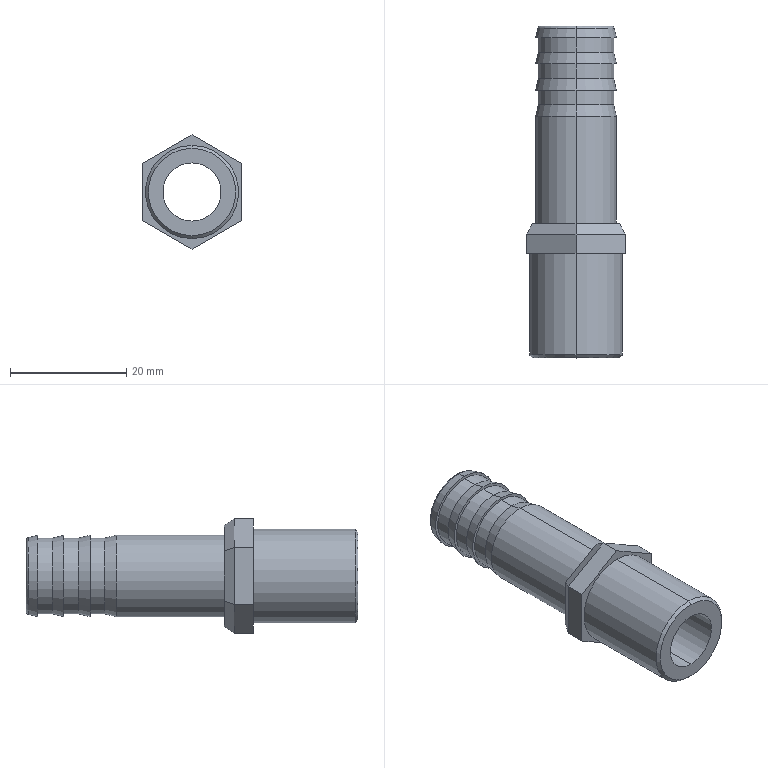Part | SolidWorks | features ICE 3, Chamfer 2, Extrusion 1, Fillet 1, RevCut 1 | 1 solid | 43 faces | box 17 x 57 x 19.63 mm | volume 5326 mm3 | plane 19 | cylinder 12 | cone 10 | torus 2 | commonest cylinder face diameters 13 x6 10 x2 14 x2 16 x2
STEP:
#1=CARTESIAN_POINT('',(0.,33.621,-6.595));
#2=VERTEX_POINT('',#1);
#3=CARTESIAN_POINT('',(0.,33.621,6.595));
#4=VERTEX_POINT('',#3);
#5=CARTESIAN_POINT('',(0.,33.621,0.));
#6=DIRECTION('',(0.,-1.,0.));
#7=DIRECTION('',(0.,0.,-1.));
#8=AXIS2_PLACEMENT_3D('',#5,#6,#7);
#9=CIRCLE('',#8,6.595);
#10=EDGE_CURVE('',#2,#4,#9,.T.);
#11=ORIENTED_EDGE('',*,*,#10,.F.);
#12=CARTESIAN_POINT('',(0.,34.,-6.11));
#13=VERTEX_POINT('',#12);
#14=CARTESIAN_POINT('',(0.,33.5,-6.11));
#15=DIRECTION('',(1.,0.,0.));
#16=DIRECTION('',(0.,0.,-1.));
#17=AXIS2_PLACEMENT_3D('',#14,#15,#16);
#18=CIRCLE('',#17,0.5);
#19=EDGE_CURVE('',#2,#13,#18,.T.);
#20=ORIENTED_EDGE('',*,*,#19,.T.);
#21=CARTESIAN_POINT('',(0.,34.,6.11));
#22=VERTEX_POINT('',#21);
#23=CARTESIAN_POINT('',(0.,34.,0.));
#24=DIRECTION('',(0.,1.,0.));
#25=DIRECTION('',(0.,0.,1.));
#26=AXIS2_PLACEMENT_3D('',#23,#24,#25);
#27=CIRCLE('',#26,6.11);
#28=EDGE_CURVE('',#22,#13,#27,.T.);
#29=ORIENTED_EDGE('',*,*,#28,.F.);
#30=CARTESIAN_POINT('',(0.,33.5,6.11));
#31=DIRECTION('',(-1.,0.,0.));
#32=DIRECTION('',(0.,0.,1.));
#33=AXIS2_PLACEMENT_3D('',#30,#31,#32);
#34=CIRCLE('',#33,0.5);
#35=EDGE_CURVE('',#4,#22,#34,.T.);
#36=ORIENTED_EDGE('',*,*,#35,.F.);
#37=EDGE_LOOP('',(#11,#20,#29,#36));
#38=FACE_OUTER_BOUND('',#37,.T.);
#39=CARTESIAN_POINT('',(0.,33.5,0.));
#40=DIRECTION('',(0.,1.,0.));
#41=DIRECTION('',(0.,0.,1.));
#42=AXIS2_PLACEMENT_3D('',#39,#40,#41);
#43=TOROIDAL_SURFACE('',#42,6.11,0.5);
#44=ADVANCED_FACE('',(#38),#43,.T.);
#45=CARTESIAN_POINT('',(0.,-23.,-7.5));
#46=VERTEX_POINT('',#45);
#47=CARTESIAN_POINT('',(0.,-23.,7.5));
#48=VERTEX_POINT('',#47);
#49=CARTESIAN_POINT('',(0.,-23.,0.));
#50=DIRECTION('',(0.,-1.,0.));
#51=DIRECTION('',(0.,0.,-1.));
#52=AXIS2_PLACEMENT_3D('',#49,#50,#51);
#53=CIRCLE('',#52,7.5);
#54=EDGE_CURVE('',#46,#48,#53,.T.);
#55=ORIENTED_EDGE('',*,*,#54,.F.);
#56=CARTESIAN_POINT('',(0.,-22.5,-8.));
#57=VERTEX_POINT('',#56);
#58=CARTESIAN_POINT('',(0.,-23.,-7.5));
#59=DIRECTION('',(0.,0.7071,-0.7071));
#60=VECTOR('',#59,1000.);
#61=LINE('',#58,#60);
#62=EDGE_CURVE('',#46,#57,#61,.T.);
#63=ORIENTED_EDGE('',*,*,#62,.T.);
#64=CARTESIAN_POINT('',(0.,-22.5,8.));
#65=VERTEX_POINT('',#64);
#66=CARTESIAN_POINT('',(0.,-22.5,0.));
#67=DIRECTION('',(0.,1.,0.));
#68=DIRECTION('',(0.,0.,-1.));
#69=AXIS2_PLACEMENT_3D('',#66,#67,#68);
#70=CIRCLE('',#69,8.);
#71=EDGE_CURVE('',#65,#57,#70,.T.);
#72=ORIENTED_EDGE('',*,*,#71,.F.);
#73=CARTESIAN_POINT('',(0.,-23.,7.5));
#74=DIRECTION('',(0.,0.7071,0.7071));
#75=VECTOR('',#74,1000.);
#76=LINE('',#73,#75);
#77=EDGE_CURVE('',#48,#65,#76,.T.);
#78=ORIENTED_EDGE('',*,*,#77,.F.);
#79=EDGE_LOOP('',(#55,#63,#72,#78));
#80=FACE_OUTER_BOUND('',#79,.T.);
#81=CARTESIAN_POINT('',(0.,-23.,0.));
#82=DIRECTION('',(0.,1.,0.));
#83=DIRECTION('',(0.,0.,1.));
#84=AXIS2_PLACEMENT_3D('',#81,#82,#83);
#85=CONICAL_SURFACE('',#84,7.5,0.7854);
#86=ADVANCED_FACE('',(#80),#85,.T.);
#87=CARTESIAN_POINT('',(0.,-23.,-5.));
#88=VERTEX_POINT('',#87);
#89=CARTESIAN_POINT('',(0.,-23.,5.));
#90=VERTEX_POINT('',#89);
#91=CARTESIAN_POINT('',(0.,-23.,0.));
#92=DIRECTION('',(0.,1.,0.));
#93=DIRECTION('',(0.,0.,1.));
#94=AXIS2_PLACEMENT_3D('',#91,#92,#93);
#95=CIRCLE('',#94,5.);
#96=EDGE_CURVE('',#88,#90,#95,.T.);
#97=ORIENTED_EDGE('',*,*,#96,.F.);
#98=CARTESIAN_POINT('',(0.,34.,-5.));
#99=VERTEX_POINT('',#98);
#100=CARTESIAN_POINT('',(0.,-23.,-5.));
#101=DIRECTION('',(0.,1.,0.));
#102=VECTOR('',#101,1000.);
#103=LINE('',#100,#102);
#104=EDGE_CURVE('',#88,#99,#103,.T.);
#105=ORIENTED_EDGE('',*,*,#104,.T.);
#106=CARTESIAN_POINT('',(0.,34.,5.));
#107=VERTEX_POINT('',#106);
#108=CARTESIAN_POINT('',(0.,34.,0.));
#109=DIRECTION('',(0.,1.,0.));
#110=DIRECTION('',(0.,0.,1.));
#111=AXIS2_PLACEMENT_3D('',#108,#109,#110);
#112=CIRCLE('',#111,5.);
#113=EDGE_CURVE('',#99,#107,#112,.T.);
#114=ORIENTED_EDGE('',*,*,#113,.T.);
#115=CARTESIAN_POINT('',(0.,-23.,5.));
#116=DIRECTION('',(0.,1.,0.));
#117=VECTOR('',#116,1000.);
#118=LINE('',#115,#117);
#119=EDGE_CURVE('',#90,#107,#118,.T.);
#120=ORIENTED_EDGE('',*,*,#119,.F.);
#121=EDGE_LOOP('',(#97,#105,#114,#120));
#122=FACE_OUTER_BOUND('',#121,.T.);
#123=CARTESIAN_POINT('',(0.,-23.,0.));
#124=DIRECTION('',(0.,1.,0.));
#125=DIRECTION('',(0.,0.,1.));
#126=AXIS2_PLACEMENT_3D('',#123,#124,#125);
#127=CYLINDRICAL_SURFACE('',#126,5.);
#128=ADVANCED_FACE('',(#122),#127,.F.);
#129=ORIENTED_EDGE('',*,*,#71,.T.);
#130=CARTESIAN_POINT('',(0.,-5.,-8.));
#131=VERTEX_POINT('',#130);
#132=CARTESIAN_POINT('',(0.,-23.,-8.));
#133=DIRECTION('',(0.,1.,0.));
#134=VECTOR('',#133,1000.);
#135=LINE('',#132,#134);
#136=EDGE_CURVE('',#57,#131,#135,.T.);
#137=ORIENTED_EDGE('',*,*,#136,.T.);
#138=CARTESIAN_POINT('',(0.,-5.,8.));
#139=VERTEX_POINT('',#138);
#140=CARTESIAN_POINT('',(0.,-5.,0.));
#141=DIRECTION('',(0.,-1.,0.));
#142=DIRECTION('',(0.,0.,-1.));
#143=AXIS2_PLACEMENT_3D('',#140,#141,#142);
#144=CIRCLE('',#143,8.);
#145=EDGE_CURVE('',#131,#139,#144,.T.);
#146=ORIENTED_EDGE('',*,*,#145,.T.);
#147=CARTESIAN_POINT('',(0.,-23.,8.));
#148=DIRECTION('',(0.,1.,0.));
#149=VECTOR('',#148,1000.);
#150=LINE('',#147,#149);
#151=EDGE_CURVE('',#65,#139,#150,.T.);
#152=ORIENTED_EDGE('',*,*,#151,.F.);
#153=EDGE_LOOP('',(#129,#137,#146,#152));
#154=FACE_OUTER_BOUND('',#153,.T.);
#155=CARTESIAN_POINT('',(0.,-23.,0.));
#156=DIRECTION('',(0.,1.,0.));
#157=DIRECTION('',(0.,0.,1.));
#158=AXIS2_PLACEMENT_3D('',#155,#156,#157);
#159=CYLINDRICAL_SURFACE('',#158,8.);
#160=ADVANCED_FACE('',(#154),#159,.T.);
#161=ORIENTED_EDGE('',*,*,#10,.T.);
#162=CARTESIAN_POINT('',(0.,32.,7.));
#163=VERTEX_POINT('',#162);
#164=CARTESIAN_POINT('',(0.,34.,6.5));
#165=DIRECTION('',(0.,-0.9701,0.2425));
#166=VECTOR('',#165,1000.);
#167=LINE('',#164,#166);
#168=EDGE_CURVE('',#4,#163,#167,.T.);
#169=ORIENTED_EDGE('',*,*,#168,.T.);
#170=CARTESIAN_POINT('',(0.,32.,-7.));
#171=VERTEX_POINT('',#170);
#172=CARTESIAN_POINT('',(0.,32.,0.));
#173=DIRECTION('',(0.,-1.,0.));
#174=DIRECTION('',(0.,0.,-1.));
#175=AXIS2_PLACEMENT_3D('',#172,#173,#174);
#176=CIRCLE('',#175,7.);
#177=EDGE_CURVE('',#171,#163,#176,.T.);
#178=ORIENTED_EDGE('',*,*,#177,.F.);
#179=CARTESIAN_POINT('',(0.,34.,-6.5));
#180=DIRECTION('',(0.,-0.9701,-0.2425));
#181=VECTOR('',#180,1000.);
#182=LINE('',#179,#181);
#183=EDGE_CURVE('',#2,#171,#182,.T.);
#184=ORIENTED_EDGE('',*,*,#183,.F.);
#185=EDGE_LOOP('',(#161,#169,#178,#184));
#186=FACE_OUTER_BOUND('',#185,.T.);
#187=CARTESIAN_POINT('',(0.,34.,0.));
#188=DIRECTION('',(0.,-1.,0.));
#189=DIRECTION('',(0.,0.,-1.));
#190=AXIS2_PLACEMENT_3D('',#187,#188,#189);
#191=CONICAL_SURFACE('',#190,6.5,0.245);
#192=ADVANCED_FACE('',(#186),#191,.T.);
#193=CARTESIAN_POINT('',(0.,29.5,-6.5));
#194=VERTEX_POINT('',#193);
#195=CARTESIAN_POINT('',(0.,29.5,6.5));
#196=VERTEX_POINT('',#195);
#197=CARTESIAN_POINT('',(0.,29.5,0.));
#198=DIRECTION('',(0.,-1.,0.));
#199=DIRECTION('',(0.,0.,-1.));
#200=AXIS2_PLACEMENT_3D('',#197,#198,#199);
#201=CIRCLE('',#200,6.5);
#202=EDGE_CURVE('',#194,#196,#201,.T.);
#203=ORIENTED_EDGE('',*,*,#202,.T.);
#204=CARTESIAN_POINT('',(0.,27.5,7.));
#205=VERTEX_POINT('',#204);
#206=CARTESIAN_POINT('',(0.,29.5,6.5));
#207=DIRECTION('',(0.,-0.9701,0.2425));
#208=VECTOR('',#207,1000.);
#209=LINE('',#206,#208);
#210=EDGE_CURVE('',#196,#205,#209,.T.);
#211=ORIENTED_EDGE('',*,*,#210,.T.);
#212=CARTESIAN_POINT('',(0.,27.5,-7.));
#213=VERTEX_POINT('',#212);
#214=CARTESIAN_POINT('',(0.,27.5,0.));
#215=DIRECTION('',(0.,-1.,0.));
#216=DIRECTION('',(0.,0.,-1.));
#217=AXIS2_PLACEMENT_3D('',#214,#215,#216);
#218=CIRCLE('',#217,7.);
#219=EDGE_CURVE('',#213,#205,#218,.T.);
#220=ORIENTED_EDGE('',*,*,#219,.F.);
#221=CARTESIAN_POINT('',(0.,29.5,-6.5));
#222=DIRECTION('',(0.,-0.9701,-0.2425));
#223=VECTOR('',#222,1000.);
#224=LINE('',#221,#223);
#225=EDGE_CURVE('',#194,#213,#224,.T.);
#226=ORIENTED_EDGE('',*,*,#225,.F.);
#227=EDGE_LOOP('',(#203,#211,#220,#226));
#228=FACE_OUTER_BOUND('',#227,.T.);
#229=CARTESIAN_POINT('',(0.,29.5,0.));
#230=DIRECTION('',(0.,-1.,0.));
#231=DIRECTION('',(0.,0.,-1.));
#232=AXIS2_PLACEMENT_3D('',#229,#230,#231);
#233=CONICAL_SURFACE('',#232,6.5,0.245);
#234=ADVANCED_FACE('',(#228),#233,.T.);
#235=CARTESIAN_POINT('',(0.,32.,-6.5));
#236=VERTEX_POINT('',#235);
#237=CARTESIAN_POINT('',(0.,32.,6.5));
#238=VERTEX_POINT('',#237);
#239=CARTESIAN_POINT('',(0.,32.,0.));
#240=DIRECTION('',(0.,-1.,0.));
#241=DIRECTION('',(0.,0.,-1.));
#242=AXIS2_PLACEMENT_3D('',#239,#240,#241);
#243=CIRCLE('',#242,6.5);
#244=EDGE_CURVE('',#236,#238,#243,.T.);
#245=ORIENTED_EDGE('',*,*,#244,.T.);
#246=CARTESIAN_POINT('',(0.,0.,6.5));
#247=DIRECTION('',(0.,-1.,0.));
#248=VECTOR('',#247,1000.);
#249=LINE('',#246,#248);
#250=EDGE_CURVE('',#238,#196,#249,.T.);
#251=ORIENTED_EDGE('',*,*,#250,.T.);
#252=ORIENTED_EDGE('',*,*,#202,.F.);
#253=CARTESIAN_POINT('',(0.,0.,-6.5));
#254=DIRECTION('',(0.,-1.,0.));
#255=VECTOR('',#254,1000.);
#256=LINE('',#253,#255);
#257=EDGE_CURVE('',#236,#194,#256,.T.);
#258=ORIENTED_EDGE('',*,*,#257,.F.);
#259=EDGE_LOOP('',(#245,#251,#252,#258));
#260=FACE_OUTER_BOUND('',#259,.T.);
#261=CARTESIAN_POINT('',(0.,0.,0.));
#262=DIRECTION('',(0.,-1.,0.));
#263=DIRECTION('',(0.,0.,-1.));
#264=AXIS2_PLACEMENT_3D('',#261,#262,#263);
#265=CYLINDRICAL_SURFACE('',#264,6.5);
#266=ADVANCED_FACE('',(#260),#265,.T.);
#267=CARTESIAN_POINT('',(0.,25.,-6.5));
#268=VERTEX_POINT('',#267);
#269=CARTESIAN_POINT('',(0.,25.,6.5));
#270=VERTEX_POINT('',#269);
#271=CARTESIAN_POINT('',(0.,25.,0.));
#272=DIRECTION('',(0.,-1.,0.));
#273=DIRECTION('',(0.,0.,-1.));
#274=AXIS2_PLACEMENT_3D('',#271,#272,#273);
#275=CIRCLE('',#274,6.5);
#276=EDGE_CURVE('',#268,#270,#275,.T.);
#277=ORIENTED_EDGE('',*,*,#276,.T.);
#278=CARTESIAN_POINT('',(0.,23.,7.));
#279=VERTEX_POINT('',#278);
#280=CARTESIAN_POINT('',(0.,25.,6.5));
#281=DIRECTION('',(0.,-0.9701,0.2425));
#282=VECTOR('',#281,1000.);
#283=LINE('',#280,#282);
#284=EDGE_CURVE('',#270,#279,#283,.T.);
#285=ORIENTED_EDGE('',*,*,#284,.T.);
#286=CARTESIAN_POINT('',(0.,23.,-7.));
#287=VERTEX_POINT('',#286);
#288=CARTESIAN_POINT('',(0.,23.,0.));
#289=DIRECTION('',(0.,-1.,0.));
#290=DIRECTION('',(0.,0.,-1.));
#291=AXIS2_PLACEMENT_3D('',#288,#289,#290);
#292=CIRCLE('',#291,7.);
#293=EDGE_CURVE('',#287,#279,#292,.T.);
#294=ORIENTED_EDGE('',*,*,#293,.F.);
#295=CARTESIAN_POINT('',(0.,25.,-6.5));
#296=DIRECTION('',(0.,-0.9701,-0.2425));
#297=VECTOR('',#296,1000.);
#298=LINE('',#295,#297);
#299=EDGE_CURVE('',#268,#287,#298,.T.);
#300=ORIENTED_EDGE('',*,*,#299,.F.);
#301=EDGE_LOOP('',(#277,#285,#294,#300));
#302=FACE_OUTER_BOUND('',#301,.T.);
#303=CARTESIAN_POINT('',(0.,25.,0.));
#304=DIRECTION('',(0.,-1.,0.));
#305=DIRECTION('',(0.,0.,-1.));
#306=AXIS2_PLACEMENT_3D('',#303,#304,#305);
#307=CONICAL_SURFACE('',#306,6.5,0.245);
#308=ADVANCED_FACE('',(#302),#307,.T.);
#309=CARTESIAN_POINT('',(0.,27.5,-6.5));
#310=VERTEX_POINT('',#309);
#311=CARTESIAN_POINT('',(0.,27.5,6.5));
#312=VERTEX_POINT('',#311);
#313=CARTESIAN_POINT('',(0.,27.5,0.));
#314=DIRECTION('',(0.,-1.,0.));
#315=DIRECTION('',(0.,0.,-1.));
#316=AXIS2_PLACEMENT_3D('',#313,#314,#315);
#317=CIRCLE('',#316,6.5);
#318=EDGE_CURVE('',#310,#312,#317,.T.);
#319=ORIENTED_EDGE('',*,*,#318,.T.);
#320=CARTESIAN_POINT('',(0.,0.,6.5));
#321=DIRECTION('',(0.,-1.,0.));
#322=VECTOR('',#321,1000.);
#323=LINE('',#320,#322);
#324=EDGE_CURVE('',#312,#270,#323,.T.);
#325=ORIENTED_EDGE('',*,*,#324,.T.);
#326=ORIENTED_EDGE('',*,*,#276,.F.);
#327=CARTESIAN_POINT('',(0.,0.,-6.5));
#328=DIRECTION('',(0.,-1.,0.));
#329=VECTOR('',#328,1000.);
#330=LINE('',#327,#329);
#331=EDGE_CURVE('',#310,#268,#330,.T.);
#332=ORIENTED_EDGE('',*,*,#331,.F.);
#333=EDGE_LOOP('',(#319,#325,#326,#332));
#334=FACE_OUTER_BOUND('',#333,.T.);
#335=CARTESIAN_POINT('',(0.,0.,0.));
#336=DIRECTION('',(0.,-1.,0.));
#337=DIRECTION('',(0.,0.,-1.));
#338=AXIS2_PLACEMENT_3D('',#335,#336,#337);
#339=CYLINDRICAL_SURFACE('',#338,6.5);
#340=ADVANCED_FACE('',(#334),#339,.T.);
#341=CARTESIAN_POINT('',(0.,18.5,-7.));
#342=VERTEX_POINT('',#341);
#343=CARTESIAN_POINT('',(0.,18.5,7.));
#344=VERTEX_POINT('',#343);
#345=CARTESIAN_POINT('',(0.,18.5,0.));
#346=DIRECTION('',(0.,-1.,0.));
#347=DIRECTION('',(0.,0.,-1.));
#348=AXIS2_PLACEMENT_3D('',#345,#346,#347);
#349=CIRCLE('',#348,7.);
#350=EDGE_CURVE('',#342,#344,#349,.T.);
#351=ORIENTED_EDGE('',*,*,#350,.T.);
#352=CARTESIAN_POINT('',(0.,0.,7.));
#353=VERTEX_POINT('',#352);
#354=CARTESIAN_POINT('',(0.,34.,7.));
#355=DIRECTION('',(0.,-1.,0.));
#356=VECTOR('',#355,1000.);
#357=LINE('',#354,#356);
#358=EDGE_CURVE('',#344,#353,#357,.T.);
#359=ORIENTED_EDGE('',*,*,#358,.T.);
#360=CARTESIAN_POINT('',(0.,0.,-7.));
#361=VERTEX_POINT('',#360);
#362=CARTESIAN_POINT('',(0.,0.,0.));
#363=DIRECTION('',(0.,1.,0.));
#364=DIRECTION('',(0.,0.,1.));
#365=AXIS2_PLACEMENT_3D('',#362,#363,#364);
#366=CIRCLE('',#365,7.);
#367=EDGE_CURVE('',#353,#361,#366,.T.);
#368=ORIENTED_EDGE('',*,*,#367,.T.);
#369=CARTESIAN_POINT('',(0.,34.,-7.));
#370=DIRECTION('',(0.,-1.,0.));
#371=VECTOR('',#370,1000.);
#372=LINE('',#369,#371);
#373=EDGE_CURVE('',#342,#361,#372,.T.);
#374=ORIENTED_EDGE('',*,*,#373,.F.);
#375=EDGE_LOOP('',(#351,#359,#368,#374));
#376=FACE_OUTER_BOUND('',#375,.T.);
#377=CARTESIAN_POINT('',(0.,34.,0.));
#378=DIRECTION('',(0.,-1.,0.));
#379=DIRECTION('',(0.,0.,-1.));
#380=AXIS2_PLACEMENT_3D('',#377,#378,#379);
#381=CYLINDRICAL_SURFACE('',#380,7.);
#382=ADVANCED_FACE('',(#376),#381,.T.);
#383=CARTESIAN_POINT('',(0.,20.5,-6.5));
#384=VERTEX_POINT('',#383);
#385=CARTESIAN_POINT('',(0.,20.5,6.5));
#386=VERTEX_POINT('',#385);
#387=CARTESIAN_POINT('',(0.,20.5,0.));
#388=DIRECTION('',(0.,-1.,0.));
#389=DIRECTION('',(0.,0.,-1.));
#390=AXIS2_PLACEMENT_3D('',#387,#388,#389);
#391=CIRCLE('',#390,6.5);
#392=EDGE_CURVE('',#384,#386,#391,.T.);
#393=ORIENTED_EDGE('',*,*,#392,.T.);
#394=CARTESIAN_POINT('',(0.,20.5,6.5));
#395=DIRECTION('',(0.,-0.9701,0.2425));
#396=VECTOR('',#395,1000.);
#397=LINE('',#394,#396);
#398=EDGE_CURVE('',#386,#344,#397,.T.);
#399=ORIENTED_EDGE('',*,*,#398,.T.);
#400=ORIENTED_EDGE('',*,*,#350,.F.);
#401=CARTESIAN_POINT('',(0.,20.5,-6.5));
#402=DIRECTION('',(0.,-0.9701,-0.2425));
#403=VECTOR('',#402,1000.);
#404=LINE('',#401,#403);
#405=EDGE_CURVE('',#384,#342,#404,.T.);
#406=ORIENTED_EDGE('',*,*,#405,.F.);
#407=EDGE_LOOP('',(#393,#399,#400,#406));
#408=FACE_OUTER_BOUND('',#407,.T.);
#409=CARTESIAN_POINT('',(0.,20.5,0.));
#410=DIRECTION('',(0.,-1.,0.));
#411=DIRECTION('',(0.,0.,-1.));
#412=AXIS2_PLACEMENT_3D('',#409,#410,#411);
#413=CONICAL_SURFACE('',#412,6.5,0.245);
#414=ADVANCED_FACE('',(#408),#413,.T.);
#415=CARTESIAN_POINT('',(0.,23.,-6.5));
#416=VERTEX_POINT('',#415);
#417=CARTESIAN_POINT('',(0.,23.,6.5));
#418=VERTEX_POINT('',#417);
#419=CARTESIAN_POINT('',(0.,23.,0.));
#420=DIRECTION('',(0.,-1.,0.));
#421=DIRECTION('',(0.,0.,-1.));
#422=AXIS2_PLACEMENT_3D('',#419,#420,#421);
#423=CIRCLE('',#422,6.5);
#424=EDGE_CURVE('',#416,#418,#423,.T.);
#425=ORIENTED_EDGE('',*,*,#424,.T.);
#426=CARTESIAN_POINT('',(0.,0.,6.5));
#427=DIRECTION('',(0.,-1.,0.));
#428=VECTOR('',#427,1000.);
#429=LINE('',#426,#428);
#430=EDGE_CURVE('',#418,#386,#429,.T.);
#431=ORIENTED_EDGE('',*,*,#430,.T.);
#432=ORIENTED_EDGE('',*,*,#392,.F.);
#433=CARTESIAN_POINT('',(0.,0.,-6.5));
#434=DIRECTION('',(0.,-1.,0.));
#435=VECTOR('',#434,1000.);
#436=LINE('',#433,#435);
#437=EDGE_CURVE('',#416,#384,#436,.T.);
#438=ORIENTED_EDGE('',*,*,#437,.F.);
#439=EDGE_LOOP('',(#425,#431,#432,#438));
#440=FACE_OUTER_BOUND('',#439,.T.);
#441=CARTESIAN_POINT('',(0.,0.,0.));
#442=DIRECTION('',(0.,-1.,0.));
#443=DIRECTION('',(0.,0.,-1.));
#444=AXIS2_PLACEMENT_3D('',#441,#442,#443);
#445=CYLINDRICAL_SURFACE('',#444,6.5);
#446=ADVANCED_FACE('',(#440),#445,.T.);
#447=ORIENTED_EDGE('',*,*,#430,.F.);
#448=CARTESIAN_POINT('',(0.,23.,0.));
#449=DIRECTION('',(0.,-1.,0.));
#450=DIRECTION('',(0.,0.,-1.));
#451=AXIS2_PLACEMENT_3D('',#448,#449,#450);
#452=CIRCLE('',#451,6.5);
#453=EDGE_CURVE('',#418,#416,#452,.T.);
#454=ORIENTED_EDGE('',*,*,#453,.T.);
#455=ORIENTED_EDGE('',*,*,#437,.T.);
#456=CARTESIAN_POINT('',(0.,20.5,0.));
#457=DIRECTION('',(0.,-1.,0.));
#458=DIRECTION('',(0.,0.,-1.));
#459=AXIS2_PLACEMENT_3D('',#456,#457,#458);
#460=CIRCLE('',#459,6.5);
#461=EDGE_CURVE('',#386,#384,#460,.T.);
#462=ORIENTED_EDGE('',*,*,#461,.F.);
#463=EDGE_LOOP('',(#447,#454,#455,#462));
#464=FACE_OUTER_BOUND('',#463,.T.);
#465=CARTESIAN_POINT('',(0.,0.,0.));
#466=DIRECTION('',(0.,-1.,0.));
#467=DIRECTION('',(0.,0.,-1.));
#468=AXIS2_PLACEMENT_3D('',#465,#466,#467);
#469=CYLINDRICAL_SURFACE('',#468,6.5);
#470=ADVANCED_FACE('',(#464),#469,.T.);
#471=ORIENTED_EDGE('',*,*,#398,.F.);
#472=ORIENTED_EDGE('',*,*,#461,.T.);
#473=ORIENTED_EDGE('',*,*,#405,.T.);
#474=CARTESIAN_POINT('',(0.,18.5,0.));
#475=DIRECTION('',(0.,-1.,0.));
#476=DIRECTION('',(0.,0.,-1.));
#477=AXIS2_PLACEMENT_3D('',#474,#475,#476);
#478=CIRCLE('',#477,7.);
#479=EDGE_CURVE('',#344,#342,#478,.T.);
#480=ORIENTED_EDGE('',*,*,#479,.F.);
#481=EDGE_LOOP('',(#471,#472,#473,#480));
#482=FACE_OUTER_BOUND('',#481,.T.);
#483=CARTESIAN_POINT('',(0.,20.5,0.));
#484=DIRECTION('',(0.,-1.,0.));
#485=DIRECTION('',(0.,0.,-1.));
#486=AXIS2_PLACEMENT_3D('',#483,#484,#485);
#487=CONICAL_SURFACE('',#486,6.5,0.245);
#488=ADVANCED_FACE('',(#482),#487,.T.);
#489=ORIENTED_EDGE('',*,*,#424,.F.);
#490=ORIENTED_EDGE('',*,*,#453,.F.);
#491=EDGE_LOOP('',(#489,#490));
#492=FACE_BOUND('',#491,.T.);
#493=ORIENTED_EDGE('',*,*,#293,.T.);
#494=CARTESIAN_POINT('',(0.,23.,0.));
#495=DIRECTION('',(0.,-1.,0.));
#496=DIRECTION('',(0.,0.,-1.));
#497=AXIS2_PLACEMENT_3D('',#494,#495,#496);
#498=CIRCLE('',#497,7.);
#499=EDGE_CURVE('',#279,#287,#498,.T.);
#500=ORIENTED_EDGE('',*,*,#499,.T.);
#501=EDGE_LOOP('',(#493,#500));
#502=FACE_OUTER_BOUND('',#501,.T.);
#503=CARTESIAN_POINT('',(0.,23.,0.));
#504=DIRECTION('',(0.,1.,0.));
#505=DIRECTION('',(0.,0.,1.));
#506=AXIS2_PLACEMENT_3D('',#503,#504,#505);
#507=PLANE('',#506);
#508=ADVANCED_FACE('',(#492,#502),#507,.F.);
#509=ORIENTED_EDGE('',*,*,#358,.F.);
#510=ORIENTED_EDGE('',*,*,#479,.T.);
#511=ORIENTED_EDGE('',*,*,#373,.T.);
#512=CARTESIAN_POINT('',(0.,0.,0.));
#513=DIRECTION('',(0.,1.,0.));
#514=DIRECTION('',(0.,0.,1.));
#515=AXIS2_PLACEMENT_3D('',#512,#513,#514);
#516=CIRCLE('',#515,7.);
#517=EDGE_CURVE('',#361,#353,#516,.T.);
#518=ORIENTED_EDGE('',*,*,#517,.T.);
#519=EDGE_LOOP('',(#509,#510,#511,#518));
#520=FACE_OUTER_BOUND('',#519,.T.);
#521=CARTESIAN_POINT('',(0.,34.,0.));
#522=DIRECTION('',(0.,-1.,0.));
#523=DIRECTION('',(0.,0.,-1.));
#524=AXIS2_PLACEMENT_3D('',#521,#522,#523);
#525=CYLINDRICAL_SURFACE('',#524,7.);
#526=ADVANCED_FACE('',(#520),#525,.T.);
#527=ORIENTED_EDGE('',*,*,#324,.F.);
#528=CARTESIAN_POINT('',(0.,27.5,0.));
#529=DIRECTION('',(0.,-1.,0.));
#530=DIRECTION('',(0.,0.,-1.));
#531=AXIS2_PLACEMENT_3D('',#528,#529,#530);
#532=CIRCLE('',#531,6.5);
#533=EDGE_CURVE('',#312,#310,#532,.T.);
#534=ORIENTED_EDGE('',*,*,#533,.T.);
#535=ORIENTED_EDGE('',*,*,#331,.T.);
#536=CARTESIAN_POINT('',(0.,25.,0.));
#537=DIRECTION('',(0.,-1.,0.));
#538=DIRECTION('',(0.,0.,-1.));
#539=AXIS2_PLACEMENT_3D('',#536,#537,#538);
#540=CIRCLE('',#539,6.5);
#541=EDGE_CURVE('',#270,#268,#540,.T.);
#542=ORIENTED_EDGE('',*,*,#541,.F.);
#543=EDGE_LOOP('',(#527,#534,#535,#542));
#544=FACE_OUTER_BOUND('',#543,.T.);
#545=CARTESIAN_POINT('',(0.,0.,0.));
#546=DIRECTION('',(0.,-1.,0.));
#547=DIRECTION('',(0.,0.,-1.));
#548=AXIS2_PLACEMENT_3D('',#545,#546,#547);
#549=CYLINDRICAL_SURFACE('',#548,6.5);
#550=ADVANCED_FACE('',(#544),#549,.T.);
#551=ORIENTED_EDGE('',*,*,#284,.F.);
#552=ORIENTED_EDGE('',*,*,#541,.T.);
#553=ORIENTED_EDGE('',*,*,#299,.T.);
#554=ORIENTED_EDGE('',*,*,#499,.F.);
#555=EDGE_LOOP('',(#551,#552,#553,#554));
#556=FACE_OUTER_BOUND('',#555,.T.);
#557=CARTESIAN_POINT('',(0.,25.,0.));
#558=DIRECTION('',(0.,-1.,0.));
#559=DIRECTION('',(0.,0.,-1.));
#560=AXIS2_PLACEMENT_3D('',#557,#558,#559);
#561=CONICAL_SURFACE('',#560,6.5,0.245);
#562=ADVANCED_FACE('',(#556),#561,.T.);
#563=ORIENTED_EDGE('',*,*,#318,.F.);
#564=ORIENTED_EDGE('',*,*,#533,.F.);
#565=EDGE_LOOP('',(#563,#564));
#566=FACE_BOUND('',#565,.T.);
#567=ORIENTED_EDGE('',*,*,#219,.T.);
#568=CARTESIAN_POINT('',(0.,27.5,0.));
#569=DIRECTION('',(0.,-1.,0.));
#570=DIRECTION('',(0.,0.,-1.));
#571=AXIS2_PLACEMENT_3D('',#568,#569,#570);
#572=CIRCLE('',#571,7.);
#573=EDGE_CURVE('',#205,#213,#572,.T.);
#574=ORIENTED_EDGE('',*,*,#573,.T.);
#575=EDGE_LOOP('',(#567,#574));
#576=FACE_OUTER_BOUND('',#575,.T.);
#577=CARTESIAN_POINT('',(0.,27.5,0.));
#578=DIRECTION('',(0.,1.,0.));
#579=DIRECTION('',(0.,0.,1.));
#580=AXIS2_PLACEMENT_3D('',#577,#578,#579);
#581=PLANE('',#580);
#582=ADVANCED_FACE('',(#566,#576),#581,.F.);
#583=ORIENTED_EDGE('',*,*,#244,.F.);
#584=CARTESIAN_POINT('',(0.,32.,0.));
#585=DIRECTION('',(0.,-1.,0.));
#586=DIRECTION('',(0.,0.,-1.));
#587=AXIS2_PLACEMENT_3D('',#584,#585,#586);
#588=CIRCLE('',#587,6.5);
#589=EDGE_CURVE('',#238,#236,#588,.T.);
#590=ORIENTED_EDGE('',*,*,#589,.F.);
#591=EDGE_LOOP('',(#583,#590));
#592=FACE_BOUND('',#591,.T.);
#593=ORIENTED_EDGE('',*,*,#177,.T.);
#594=CARTESIAN_POINT('',(0.,32.,0.));
#595=DIRECTION('',(0.,-1.,0.));
#596=DIRECTION('',(0.,0.,-1.));
#597=AXIS2_PLACEMENT_3D('',#594,#595,#596);
#598=CIRCLE('',#597,7.);
#599=EDGE_CURVE('',#163,#171,#598,.T.);
#600=ORIENTED_EDGE('',*,*,#599,.T.);
#601=EDGE_LOOP('',(#593,#600));
#602=FACE_OUTER_BOUND('',#601,.T.);
#603=CARTESIAN_POINT('',(0.,32.,0.));
#604=DIRECTION('',(0.,1.,0.));
#605=DIRECTION('',(0.,0.,1.));
#606=AXIS2_PLACEMENT_3D('',#603,#604,#605);
#607=PLANE('',#606);
#608=ADVANCED_FACE('',(#592,#602),#607,.F.);
#609=ORIENTED_EDGE('',*,*,#250,.F.);
#610=ORIENTED_EDGE('',*,*,#589,.T.);
#611=ORIENTED_EDGE('',*,*,#257,.T.);
#612=CARTESIAN_POINT('',(0.,29.5,0.));
#613=DIRECTION('',(0.,-1.,0.));
#614=DIRECTION('',(0.,0.,-1.));
#615=AXIS2_PLACEMENT_3D('',#612,#613,#614);
#616=CIRCLE('',#615,6.5);
#617=EDGE_CURVE('',#196,#194,#616,.T.);
#618=ORIENTED_EDGE('',*,*,#617,.F.);
#619=EDGE_LOOP('',(#609,#610,#611,#618));
#620=FACE_OUTER_BOUND('',#619,.T.);
#621=CARTESIAN_POINT('',(0.,0.,0.));
#622=DIRECTION('',(0.,-1.,0.));
#623=DIRECTION('',(0.,0.,-1.));
#624=AXIS2_PLACEMENT_3D('',#621,#622,#623);
#625=CYLINDRICAL_SURFACE('',#624,6.5);
#626=ADVANCED_FACE('',(#620),#625,.T.);
#627=ORIENTED_EDGE('',*,*,#210,.F.);
#628=ORIENTED_EDGE('',*,*,#617,.T.);
#629=ORIENTED_EDGE('',*,*,#225,.T.);
#630=ORIENTED_EDGE('',*,*,#573,.F.);
#631=EDGE_LOOP('',(#627,#628,#629,#630));
#632=FACE_OUTER_BOUND('',#631,.T.);
#633=CARTESIAN_POINT('',(0.,29.5,0.));
#634=DIRECTION('',(0.,-1.,0.));
#635=DIRECTION('',(0.,0.,-1.));
#636=AXIS2_PLACEMENT_3D('',#633,#634,#635);
#637=CONICAL_SURFACE('',#636,6.5,0.245);
#638=ADVANCED_FACE('',(#632),#637,.T.);
#639=ORIENTED_EDGE('',*,*,#168,.F.);
#640=CARTESIAN_POINT('',(0.,33.621,0.));
#641=DIRECTION('',(0.,-1.,0.));
#642=DIRECTION('',(0.,0.,-1.));
#643=AXIS2_PLACEMENT_3D('',#640,#641,#642);
#644=CIRCLE('',#643,6.595);
#645=EDGE_CURVE('',#4,#2,#644,.T.);
#646=ORIENTED_EDGE('',*,*,#645,.T.);
#647=ORIENTED_EDGE('',*,*,#183,.T.);
#648=ORIENTED_EDGE('',*,*,#599,.F.);
#649=EDGE_LOOP('',(#639,#646,#647,#648));
#650=FACE_OUTER_BOUND('',#649,.T.);
#651=CARTESIAN_POINT('',(0.,34.,0.));
#652=DIRECTION('',(0.,-1.,0.));
#653=DIRECTION('',(0.,0.,-1.));
#654=AXIS2_PLACEMENT_3D('',#651,#652,#653);
#655=CONICAL_SURFACE('',#654,6.5,0.245);
#656=ADVANCED_FACE('',(#650),#655,.T.);
#657=ORIENTED_EDGE('',*,*,#28,.T.);
#658=CARTESIAN_POINT('',(0.,34.,0.));
#659=DIRECTION('',(0.,1.,0.));
#660=DIRECTION('',(0.,0.,1.));
#661=AXIS2_PLACEMENT_3D('',#658,#659,#660);
#662=CIRCLE('',#661,6.11);
#663=EDGE_CURVE('',#13,#22,#662,.T.);
#664=ORIENTED_EDGE('',*,*,#663,.T.);
#665=EDGE_LOOP('',(#657,#664));
#666=FACE_OUTER_BOUND('',#665,.T.);
#667=CARTESIAN_POINT('',(0.,34.,0.));
#668=DIRECTION('',(0.,1.,0.));
#669=DIRECTION('',(0.,0.,1.));
#670=AXIS2_PLACEMENT_3D('',#667,#668,#669);
#671=CIRCLE('',#670,5.);
#672=EDGE_CURVE('',#107,#99,#671,.T.);
#673=ORIENTED_EDGE('',*,*,#672,.F.);
#674=ORIENTED_EDGE('',*,*,#113,.F.);
#675=EDGE_LOOP('',(#673,#674));
#676=FACE_BOUND('',#675,.T.);
#677=CARTESIAN_POINT('',(0.,34.,0.));
#678=DIRECTION('',(0.,1.,0.));
#679=DIRECTION('',(0.,0.,1.));
#680=AXIS2_PLACEMENT_3D('',#677,#678,#679);
#681=PLANE('',#680);
#682=ADVANCED_FACE('',(#666,#676),#681,.T.);
#683=CARTESIAN_POINT('',(0.,-5.,-9.815));
#684=VERTEX_POINT('',#683);
#685=CARTESIAN_POINT('',(0.,-1.732,-9.815));
#686=VERTEX_POINT('',#685);
#687=CARTESIAN_POINT('',(0.,-5.,-9.815));
#688=DIRECTION('',(0.,1.,0.));
#689=VECTOR('',#688,1000.);
#690=LINE('',#687,#689);
#691=EDGE_CURVE('',#684,#686,#690,.T.);
#692=ORIENTED_EDGE('',*,*,#691,.T.);
#693=CARTESIAN_POINT('',(8.5,-1.732,-4.907));
#694=VERTEX_POINT('',#693);
#695=CARTESIAN_POINT('',(0.,-1.732,-9.815));
#696=DIRECTION('',(0.866,0.,0.5));
#697=VECTOR('',#696,1000.);
#698=LINE('',#695,#697);
#699=EDGE_CURVE('',#686,#694,#698,.T.);
#700=ORIENTED_EDGE('',*,*,#699,.T.);
#701=CARTESIAN_POINT('',(8.5,-5.,-4.907));
#702=VERTEX_POINT('',#701);
#703=CARTESIAN_POINT('',(8.5,-5.,-4.907));
#704=DIRECTION('',(0.,1.,0.));
#705=VECTOR('',#704,1000.);
#706=LINE('',#703,#705);
#707=EDGE_CURVE('',#702,#694,#706,.T.);
#708=ORIENTED_EDGE('',*,*,#707,.F.);
#709=CARTESIAN_POINT('',(0.,-5.,-9.815));
#710=DIRECTION('',(0.866,0.,0.5));
#711=VECTOR('',#710,1000.);
#712=LINE('',#709,#711);
#713=EDGE_CURVE('',#684,#702,#712,.T.);
#714=ORIENTED_EDGE('',*,*,#713,.F.);
#715=EDGE_LOOP('',(#692,#700,#708,#714));
#716=FACE_OUTER_BOUND('',#715,.T.);
#717=CARTESIAN_POINT('',(0.,-5.,-9.815));
#718=DIRECTION('',(-0.5,0.,0.866));
#719=DIRECTION('',(0.866,0.,0.5));
#720=AXIS2_PLACEMENT_3D('',#717,#718,#719);
#721=PLANE('',#720);
#722=ADVANCED_FACE('',(#716),#721,.F.);
#723=ORIENTED_EDGE('',*,*,#707,.T.);
#724=CARTESIAN_POINT('',(8.5,-1.732,4.907));
#725=VERTEX_POINT('',#724);
#726=CARTESIAN_POINT('',(8.5,-1.732,-4.907));
#727=DIRECTION('',(0.,0.,1.));
#728=VECTOR('',#727,1000.);
#729=LINE('',#726,#728);
#730=EDGE_CURVE('',#694,#725,#729,.T.);
#731=ORIENTED_EDGE('',*,*,#730,.T.);
#732=CARTESIAN_POINT('',(8.5,-5.,4.907));
#733=VERTEX_POINT('',#732);
#734=CARTESIAN_POINT('',(8.5,-5.,4.907));
#735=DIRECTION('',(0.,1.,0.));
#736=VECTOR('',#735,1000.);
#737=LINE('',#734,#736);
#738=EDGE_CURVE('',#733,#725,#737,.T.);
#739=ORIENTED_EDGE('',*,*,#738,.F.);
#740=CARTESIAN_POINT('',(8.5,-5.,-4.907));
#741=DIRECTION('',(0.,0.,1.));
#742=VECTOR('',#741,1000.);
#743=LINE('',#740,#742);
#744=EDGE_CURVE('',#702,#733,#743,.T.);
#745=ORIENTED_EDGE('',*,*,#744,.F.);
#746=EDGE_LOOP('',(#723,#731,#739,#745));
#747=FACE_OUTER_BOUND('',#746,.T.);
#748=CARTESIAN_POINT('',(8.5,-5.,-4.907));
#749=DIRECTION('',(-1.,0.,0.));
#750=DIRECTION('',(0.,0.,1.));
#751=AXIS2_PLACEMENT_3D('',#748,#749,#750);
#752=PLANE('',#751);
#753=ADVANCED_FACE('',(#747),#752,.F.);
#754=ORIENTED_EDGE('',*,*,#738,.T.);
#755=CARTESIAN_POINT('',(0.,-1.732,9.815));
#756=VERTEX_POINT('',#755);
#757=CARTESIAN_POINT('',(8.5,-1.732,4.907));
#758=DIRECTION('',(-0.866,0.,0.5));
#759=VECTOR('',#758,1000.);
#760=LINE('',#757,#759);
#761=EDGE_CURVE('',#725,#756,#760,.T.);
#762=ORIENTED_EDGE('',*,*,#761,.T.);
#763=CARTESIAN_POINT('',(0.,-5.,9.815));
#764=VERTEX_POINT('',#763);
#765=CARTESIAN_POINT('',(0.,-5.,9.815));
#766=DIRECTION('',(0.,1.,0.));
#767=VECTOR('',#766,1000.);
#768=LINE('',#765,#767);
#769=EDGE_CURVE('',#764,#756,#768,.T.);
#770=ORIENTED_EDGE('',*,*,#769,.F.);
#771=CARTESIAN_POINT('',(8.5,-5.,4.907));
#772=DIRECTION('',(-0.866,0.,0.5));
#773=VECTOR('',#772,1000.);
#774=LINE('',#771,#773);
#775=EDGE_CURVE('',#733,#764,#774,.T.);
#776=ORIENTED_EDGE('',*,*,#775,.F.);
#777=EDGE_LOOP('',(#754,#762,#770,#776));
#778=FACE_OUTER_BOUND('',#777,.T.);
#779=CARTESIAN_POINT('',(8.5,-5.,4.907));
#780=DIRECTION('',(-0.5,0.,-0.866));
#781=DIRECTION('',(-0.866,0.,0.5));
#782=AXIS2_PLACEMENT_3D('',#779,#780,#781);
#783=PLANE('',#782);
#784=ADVANCED_FACE('',(#778),#783,.F.);
#785=ORIENTED_EDGE('',*,*,#769,.T.);
#786=CARTESIAN_POINT('',(-8.5,-1.732,4.907));
#787=VERTEX_POINT('',#786);
#788=CARTESIAN_POINT('',(0.,-1.732,9.815));
#789=DIRECTION('',(-0.866,0.,-0.5));
#790=VECTOR('',#789,1000.);
#791=LINE('',#788,#790);
#792=EDGE_CURVE('',#756,#787,#791,.T.);
#793=ORIENTED_EDGE('',*,*,#792,.T.);
#794=CARTESIAN_POINT('',(-8.5,-5.,4.907));
#795=VERTEX_POINT('',#794);
#796=CARTESIAN_POINT('',(-8.5,-5.,4.907));
#797=DIRECTION('',(0.,1.,0.));
#798=VECTOR('',#797,1000.);
#799=LINE('',#796,#798);
#800=EDGE_CURVE('',#795,#787,#799,.T.);
#801=ORIENTED_EDGE('',*,*,#800,.F.);
#802=CARTESIAN_POINT('',(0.,-5.,9.815));
#803=DIRECTION('',(-0.866,0.,-0.5));
#804=VECTOR('',#803,1000.);
#805=LINE('',#802,#804);
#806=EDGE_CURVE('',#764,#795,#805,.T.);
#807=ORIENTED_EDGE('',*,*,#806,.F.);
#808=EDGE_LOOP('',(#785,#793,#801,#807));
#809=FACE_OUTER_BOUND('',#808,.T.);
#810=CARTESIAN_POINT('',(0.,-5.,9.815));
#811=DIRECTION('',(0.5,0.,-0.866));
#812=DIRECTION('',(-0.866,0.,-0.5));
#813=AXIS2_PLACEMENT_3D('',#810,#811,#812);
#814=PLANE('',#813);
#815=ADVANCED_FACE('',(#809),#814,.F.);
#816=ORIENTED_EDGE('',*,*,#800,.T.);
#817=CARTESIAN_POINT('',(-8.5,-1.732,-4.907));
#818=VERTEX_POINT('',#817);
#819=CARTESIAN_POINT('',(-8.5,-1.732,4.907));
#820=DIRECTION('',(0.,0.,-1.));
#821=VECTOR('',#820,1000.);
#822=LINE('',#819,#821);
#823=EDGE_CURVE('',#787,#818,#822,.T.);
#824=ORIENTED_EDGE('',*,*,#823,.T.);
#825=CARTESIAN_POINT('',(-8.5,-5.,-4.907));
#826=VERTEX_POINT('',#825);
#827=CARTESIAN_POINT('',(-8.5,-5.,-4.907));
#828=DIRECTION('',(0.,1.,0.));
#829=VECTOR('',#828,1000.);
#830=LINE('',#827,#829);
#831=EDGE_CURVE('',#826,#818,#830,.T.);
#832=ORIENTED_EDGE('',*,*,#831,.F.);
#833=CARTESIAN_POINT('',(-8.5,-5.,4.907));
#834=DIRECTION('',(0.,0.,-1.));
#835=VECTOR('',#834,1000.);
#836=LINE('',#833,#835);
#837=EDGE_CURVE('',#795,#826,#836,.T.);
#838=ORIENTED_EDGE('',*,*,#837,.F.);
#839=EDGE_LOOP('',(#816,#824,#832,#838));
#840=FACE_OUTER_BOUND('',#839,.T.);
#841=CARTESIAN_POINT('',(-8.5,-5.,4.907));
#842=DIRECTION('',(1.,0.,0.));
#843=DIRECTION('',(0.,0.,-1.));
#844=AXIS2_PLACEMENT_3D('',#841,#842,#843);
#845=PLANE('',#844);
#846=ADVANCED_FACE('',(#840),#845,.F.);
#847=ORIENTED_EDGE('',*,*,#831,.T.);
#848=CARTESIAN_POINT('',(-8.5,-1.732,-4.907));
#849=DIRECTION('',(0.866,0.,-0.5));
#850=VECTOR('',#849,1000.);
#851=LINE('',#848,#850);
#852=EDGE_CURVE('',#818,#686,#851,.T.);
#853=ORIENTED_EDGE('',*,*,#852,.T.);
#854=ORIENTED_EDGE('',*,*,#691,.F.);
#855=CARTESIAN_POINT('',(-8.5,-5.,-4.907));
#856=DIRECTION('',(0.866,0.,-0.5));
#857=VECTOR('',#856,1000.);
#858=LINE('',#855,#857);
#859=EDGE_CURVE('',#826,#684,#858,.T.);
#860=ORIENTED_EDGE('',*,*,#859,.F.);
#861=EDGE_LOOP('',(#847,#853,#854,#860));
#862=FACE_OUTER_BOUND('',#861,.T.);
#863=CARTESIAN_POINT('',(-8.5,-5.,-4.907));
#864=DIRECTION('',(0.5,0.,0.866));
#865=DIRECTION('',(0.866,0.,-0.5));
#866=AXIS2_PLACEMENT_3D('',#863,#864,#865);
#867=PLANE('',#866);
#868=ADVANCED_FACE('',(#862),#867,.F.);
#869=CARTESIAN_POINT('',(0.,-5.,0.));
#870=DIRECTION('',(0.,-1.,0.));
#871=DIRECTION('',(0.,0.,-1.));
#872=AXIS2_PLACEMENT_3D('',#869,#870,#871);
#873=CIRCLE('',#872,8.);
#874=EDGE_CURVE('',#139,#131,#873,.T.);
#875=ORIENTED_EDGE('',*,*,#874,.F.);
#876=ORIENTED_EDGE('',*,*,#145,.F.);
#877=EDGE_LOOP('',(#875,#876));
#878=FACE_BOUND('',#877,.T.);
#879=ORIENTED_EDGE('',*,*,#713,.T.);
#880=ORIENTED_EDGE('',*,*,#744,.T.);
#881=ORIENTED_EDGE('',*,*,#775,.T.);
#882=ORIENTED_EDGE('',*,*,#806,.T.);
#883=ORIENTED_EDGE('',*,*,#837,.T.);
#884=ORIENTED_EDGE('',*,*,#859,.T.);
#885=EDGE_LOOP('',(#879,#880,#881,#882,#883,#884));
#886=FACE_OUTER_BOUND('',#885,.T.);
#887=CARTESIAN_POINT('',(0.,-5.,0.));
#888=DIRECTION('',(0.,-1.,0.));
#889=DIRECTION('',(0.,0.,-1.));
#890=AXIS2_PLACEMENT_3D('',#887,#888,#889);
#891=PLANE('',#890);
#892=ADVANCED_FACE('',(#878,#886),#891,.T.);
#893=CARTESIAN_POINT('',(-7.5,0.,-4.33));
#894=VERTEX_POINT('',#893);
#895=CARTESIAN_POINT('',(-7.5,0.,4.33));
#896=VERTEX_POINT('',#895);
#897=CARTESIAN_POINT('',(-7.5,0.,0.));
#898=DIRECTION('',(0.,0.,1.));
#899=VECTOR('',#898,1000.);
#900=LINE('',#897,#899);
#901=EDGE_CURVE('',#894,#896,#900,.T.);
#902=ORIENTED_EDGE('',*,*,#901,.T.);
#903=CARTESIAN_POINT('',(0.,0.,8.66));
#904=VERTEX_POINT('',#903);
#905=CARTESIAN_POINT('',(-3.75,0.,6.495));
#906=DIRECTION('',(0.866,0.,0.5));
#907=VECTOR('',#906,1000.);
#908=LINE('',#905,#907);
#909=EDGE_CURVE('',#896,#904,#908,.T.);
#910=ORIENTED_EDGE('',*,*,#909,.T.);
#911=CARTESIAN_POINT('',(7.5,0.,4.33));
#912=VERTEX_POINT('',#911);
#913=CARTESIAN_POINT('',(3.75,0.,6.495));
#914=DIRECTION('',(0.866,0.,-0.5));
#915=VECTOR('',#914,1000.);
#916=LINE('',#913,#915);
#917=EDGE_CURVE('',#904,#912,#916,.T.);
#918=ORIENTED_EDGE('',*,*,#917,.T.);
#919=CARTESIAN_POINT('',(7.5,0.,-4.33));
#920=VERTEX_POINT('',#919);
#921=CARTESIAN_POINT('',(7.5,0.,0.));
#922=DIRECTION('',(0.,0.,-1.));
#923=VECTOR('',#922,1000.);
#924=LINE('',#921,#923);
#925=EDGE_CURVE('',#912,#920,#924,.T.);
#926=ORIENTED_EDGE('',*,*,#925,.T.);
#927=CARTESIAN_POINT('',(0.,0.,-8.66));
#928=VERTEX_POINT('',#927);
#929=CARTESIAN_POINT('',(3.75,0.,-6.495));
#930=DIRECTION('',(-0.866,0.,-0.5));
#931=VECTOR('',#930,1000.);
#932=LINE('',#929,#931);
#933=EDGE_CURVE('',#920,#928,#932,.T.);
#934=ORIENTED_EDGE('',*,*,#933,.T.);
#935=CARTESIAN_POINT('',(-3.75,0.,-6.495));
#936=DIRECTION('',(-0.866,0.,0.5));
#937=VECTOR('',#936,1000.);
#938=LINE('',#935,#937);
#939=EDGE_CURVE('',#928,#894,#938,.T.);
#940=ORIENTED_EDGE('',*,*,#939,.T.);
#941=EDGE_LOOP('',(#902,#910,#918,#926,#934,#940));
#942=FACE_OUTER_BOUND('',#941,.T.);
#943=ORIENTED_EDGE('',*,*,#517,.F.);
#944=ORIENTED_EDGE('',*,*,#367,.F.);
#945=EDGE_LOOP('',(#943,#944));
#946=FACE_BOUND('',#945,.T.);
#947=CARTESIAN_POINT('',(0.,0.,0.));
#948=DIRECTION('',(0.,-1.,0.));
#949=DIRECTION('',(0.,0.,-1.));
#950=AXIS2_PLACEMENT_3D('',#947,#948,#949);
#951=PLANE('',#950);
#952=ADVANCED_FACE('',(#942,#946),#951,.F.);
#953=ORIENTED_EDGE('',*,*,#136,.F.);
#954=CARTESIAN_POINT('',(0.,-22.5,0.));
#955=DIRECTION('',(0.,1.,0.));
#956=DIRECTION('',(0.,0.,-1.));
#957=AXIS2_PLACEMENT_3D('',#954,#955,#956);
#958=CIRCLE('',#957,8.);
#959=EDGE_CURVE('',#57,#65,#958,.T.);
#960=ORIENTED_EDGE('',*,*,#959,.T.);
#961=ORIENTED_EDGE('',*,*,#151,.T.);
#962=ORIENTED_EDGE('',*,*,#874,.T.);
#963=EDGE_LOOP('',(#953,#960,#961,#962));
#964=FACE_OUTER_BOUND('',#963,.T.);
#965=CARTESIAN_POINT('',(0.,-23.,0.));
#966=DIRECTION('',(0.,1.,0.));
#967=DIRECTION('',(0.,0.,1.));
#968=AXIS2_PLACEMENT_3D('',#965,#966,#967);
#969=CYLINDRICAL_SURFACE('',#968,8.);
#970=ADVANCED_FACE('',(#964),#969,.T.);
#971=CARTESIAN_POINT('',(0.,-23.,0.));
#972=DIRECTION('',(0.,-1.,0.));
#973=DIRECTION('',(0.,0.,-1.));
#974=AXIS2_PLACEMENT_3D('',#971,#972,#973);
#975=CIRCLE('',#974,7.5);
#976=EDGE_CURVE('',#48,#46,#975,.T.);
#977=ORIENTED_EDGE('',*,*,#976,.T.);
#978=ORIENTED_EDGE('',*,*,#54,.T.);
#979=EDGE_LOOP('',(#977,#978));
#980=FACE_OUTER_BOUND('',#979,.T.);
#981=CARTESIAN_POINT('',(0.,-23.,0.));
#982=DIRECTION('',(0.,1.,0.));
#983=DIRECTION('',(0.,0.,1.));
#984=AXIS2_PLACEMENT_3D('',#981,#982,#983);
#985=CIRCLE('',#984,5.);
#986=EDGE_CURVE('',#90,#88,#985,.T.);
#987=ORIENTED_EDGE('',*,*,#986,.T.);
#988=ORIENTED_EDGE('',*,*,#96,.T.);
#989=EDGE_LOOP('',(#987,#988));
#990=FACE_BOUND('',#989,.T.);
#991=CARTESIAN_POINT('',(0.,-23.,0.));
#992=DIRECTION('',(0.,-1.,0.));
#993=DIRECTION('',(0.,0.,-1.));
#994=AXIS2_PLACEMENT_3D('',#991,#992,#993);
#995=PLANE('',#994);
#996=ADVANCED_FACE('',(#980,#990),#995,.T.);
#997=ORIENTED_EDGE('',*,*,#104,.F.);
#998=ORIENTED_EDGE('',*,*,#986,.F.);
#999=ORIENTED_EDGE('',*,*,#119,.T.);
#1000=ORIENTED_EDGE('',*,*,#672,.T.);
#1001=EDGE_LOOP('',(#997,#998,#999,#1000));
#1002=FACE_OUTER_BOUND('',#1001,.T.);
#1003=CARTESIAN_POINT('',(0.,-23.,0.));
#1004=DIRECTION('',(0.,1.,0.));
#1005=DIRECTION('',(0.,0.,1.));
#1006=AXIS2_PLACEMENT_3D('',#1003,#1004,#1005);
#1007=CYLINDRICAL_SURFACE('',#1006,5.);
#1008=ADVANCED_FACE('',(#1002),#1007,.F.);
#1009=CARTESIAN_POINT('',(0.,-1.732,-9.815));
#1010=DIRECTION('',(0.,-0.8321,-0.5547));
#1011=VECTOR('',#1010,1000.);
#1012=LINE('',#1009,#1011);
#1013=EDGE_CURVE('',#928,#686,#1012,.T.);
#1014=ORIENTED_EDGE('',*,*,#1013,.F.);
#1015=ORIENTED_EDGE('',*,*,#933,.F.);
#1016=CARTESIAN_POINT('',(8.5,-1.732,-4.907));
#1017=DIRECTION('',(-0.4804,0.8321,0.2774));
#1018=VECTOR('',#1017,1000.);
#1019=LINE('',#1016,#1018);
#1020=EDGE_CURVE('',#694,#920,#1019,.T.);
#1021=ORIENTED_EDGE('',*,*,#1020,.F.);
#1022=ORIENTED_EDGE('',*,*,#699,.F.);
#1023=EDGE_LOOP('',(#1014,#1015,#1021,#1022));
#1024=FACE_OUTER_BOUND('',#1023,.T.);
#1025=CARTESIAN_POINT('',(0.,-1.732,-9.815));
#1026=DIRECTION('',(-0.433,-0.5,0.75));
#1027=DIRECTION('',(0.866,0.,0.5));
#1028=AXIS2_PLACEMENT_3D('',#1025,#1026,#1027);
#1029=PLANE('',#1028);
#1030=ADVANCED_FACE('',(#1024),#1029,.F.);
#1031=ORIENTED_EDGE('',*,*,#1020,.T.);
#1032=ORIENTED_EDGE('',*,*,#925,.F.);
#1033=CARTESIAN_POINT('',(8.5,-1.732,4.907));
#1034=DIRECTION('',(-0.4804,0.8321,-0.2774));
#1035=VECTOR('',#1034,1000.);
#1036=LINE('',#1033,#1035);
#1037=EDGE_CURVE('',#725,#912,#1036,.T.);
#1038=ORIENTED_EDGE('',*,*,#1037,.F.);
#1039=ORIENTED_EDGE('',*,*,#730,.F.);
#1040=EDGE_LOOP('',(#1031,#1032,#1038,#1039));
#1041=FACE_OUTER_BOUND('',#1040,.T.);
#1042=CARTESIAN_POINT('',(8.5,-1.732,-4.907));
#1043=DIRECTION('',(-0.866,-0.5,0.));
#1044=DIRECTION('',(0.,0.,1.));
#1045=AXIS2_PLACEMENT_3D('',#1042,#1043,#1044);
#1046=PLANE('',#1045);
#1047=ADVANCED_FACE('',(#1041),#1046,.F.);
#1048=ORIENTED_EDGE('',*,*,#1013,.T.);
#1049=ORIENTED_EDGE('',*,*,#852,.F.);
#1050=CARTESIAN_POINT('',(-8.5,-1.732,-4.907));
#1051=DIRECTION('',(-0.4804,-0.8321,-0.2774));
#1052=VECTOR('',#1051,1000.);
#1053=LINE('',#1050,#1052);
#1054=EDGE_CURVE('',#894,#818,#1053,.T.);
#1055=ORIENTED_EDGE('',*,*,#1054,.F.);
#1056=ORIENTED_EDGE('',*,*,#939,.F.);
#1057=EDGE_LOOP('',(#1048,#1049,#1055,#1056));
#1058=FACE_OUTER_BOUND('',#1057,.T.);
#1059=CARTESIAN_POINT('',(-8.5,-1.732,-4.907));
#1060=DIRECTION('',(0.433,-0.5,0.75));
#1061=DIRECTION('',(0.866,0.,-0.5));
#1062=AXIS2_PLACEMENT_3D('',#1059,#1060,#1061);
#1063=PLANE('',#1062);
#1064=ADVANCED_FACE('',(#1058),#1063,.F.);
#1065=ORIENTED_EDGE('',*,*,#1037,.T.);
#1066=ORIENTED_EDGE('',*,*,#917,.F.);
#1067=CARTESIAN_POINT('',(0.,0.5329,8.305));
#1068=DIRECTION('',(0.,0.8321,-0.5547));
#1069=VECTOR('',#1068,1000.);
#1070=LINE('',#1067,#1069);
#1071=EDGE_CURVE('',#756,#904,#1070,.T.);
#1072=ORIENTED_EDGE('',*,*,#1071,.F.);
#1073=ORIENTED_EDGE('',*,*,#761,.F.);
#1074=EDGE_LOOP('',(#1065,#1066,#1072,#1073));
#1075=FACE_OUTER_BOUND('',#1074,.T.);
#1076=CARTESIAN_POINT('',(8.5,-1.732,4.907));
#1077=DIRECTION('',(-0.433,-0.5,-0.75));
#1078=DIRECTION('',(-0.866,0.,0.5));
#1079=AXIS2_PLACEMENT_3D('',#1076,#1077,#1078);
#1080=PLANE('',#1079);
#1081=ADVANCED_FACE('',(#1075),#1080,.F.);
#1082=ORIENTED_EDGE('',*,*,#1054,.T.);
#1083=ORIENTED_EDGE('',*,*,#823,.F.);
#1084=CARTESIAN_POINT('',(-8.5,-1.732,4.907));
#1085=DIRECTION('',(-0.4804,-0.8321,0.2774));
#1086=VECTOR('',#1085,1000.);
#1087=LINE('',#1084,#1086);
#1088=EDGE_CURVE('',#896,#787,#1087,.T.);
#1089=ORIENTED_EDGE('',*,*,#1088,.F.);
#1090=ORIENTED_EDGE('',*,*,#901,.F.);
#1091=EDGE_LOOP('',(#1082,#1083,#1089,#1090));
#1092=FACE_OUTER_BOUND('',#1091,.T.);
#1093=CARTESIAN_POINT('',(-8.5,-1.732,4.907));
#1094=DIRECTION('',(0.866,-0.5,0.));
#1095=DIRECTION('',(0.,0.,-1.));
#1096=AXIS2_PLACEMENT_3D('',#1093,#1094,#1095);
#1097=PLANE('',#1096);
#1098=ADVANCED_FACE('',(#1092),#1097,.F.);
#1099=ORIENTED_EDGE('',*,*,#1071,.T.);
#1100=ORIENTED_EDGE('',*,*,#909,.F.);
#1101=ORIENTED_EDGE('',*,*,#1088,.T.);
#1102=ORIENTED_EDGE('',*,*,#792,.F.);
#1103=EDGE_LOOP('',(#1099,#1100,#1101,#1102));
#1104=FACE_OUTER_BOUND('',#1103,.T.);
#1105=CARTESIAN_POINT('',(0.,-1.732,9.815));
#1106=DIRECTION('',(0.433,-0.5,-0.75));
#1107=DIRECTION('',(-0.866,0.,-0.5));
#1108=AXIS2_PLACEMENT_3D('',#1105,#1106,#1107);
#1109=PLANE('',#1108);
#1110=ADVANCED_FACE('',(#1104),#1109,.F.);
#1111=ORIENTED_EDGE('',*,*,#62,.F.);
#1112=ORIENTED_EDGE('',*,*,#976,.F.);
#1113=ORIENTED_EDGE('',*,*,#77,.T.);
#1114=ORIENTED_EDGE('',*,*,#959,.F.);
#1115=EDGE_LOOP('',(#1111,#1112,#1113,#1114));
#1116=FACE_OUTER_BOUND('',#1115,.T.);
#1117=CARTESIAN_POINT('',(0.,-23.,0.));
#1118=DIRECTION('',(0.,1.,0.));
#1119=DIRECTION('',(0.,0.,1.));
#1120=AXIS2_PLACEMENT_3D('',#1117,#1118,#1119);
#1121=CONICAL_SURFACE('',#1120,7.5,0.7854);
#1122=ADVANCED_FACE('',(#1116),#1121,.T.);
#1123=ORIENTED_EDGE('',*,*,#19,.F.);
#1124=ORIENTED_EDGE('',*,*,#645,.F.);
#1125=ORIENTED_EDGE('',*,*,#35,.T.);
#1126=ORIENTED_EDGE('',*,*,#663,.F.);
#1127=EDGE_LOOP('',(#1123,#1124,#1125,#1126));
#1128=FACE_OUTER_BOUND('',#1127,.T.);
#1129=CARTESIAN_POINT('',(0.,33.5,0.));
#1130=DIRECTION('',(0.,1.,0.));
#1131=DIRECTION('',(0.,0.,1.));
#1132=AXIS2_PLACEMENT_3D('',#1129,#1130,#1131);
#1133=TOROIDAL_SURFACE('',#1132,6.11,0.5);
#1134=ADVANCED_FACE('',(#1128),#1133,.T.);
#1135=CLOSED_SHELL('',(#44,#86,#128,#160,#192,#234,#266,#308,#340,#382,#414,#446,#470,#488,#508,#526,#550,#562,#582,#608,#626,#638,#656,#682,#722,#753,#784,#815,#846,#868,#892,#952,#970,#996,#1008,#1030,#1047,#1064,#1081,#1098,#1110,#1122,#1134));
#1136=MANIFOLD_SOLID_BREP('',#1135);
#1137=CARTESIAN_POINT('',(0.,0.,0.));
#1138=DIRECTION('',(0.,0.,1.));
#1139=DIRECTION('',(1.,0.,0.));
#1140=AXIS2_PLACEMENT_3D('',#1137,#1138,#1139);
#1141=(LENGTH_UNIT()NAMED_UNIT(*)SI_UNIT(.MILLI.,.METRE.));
#1142=UNCERTAINTY_MEASURE_WITH_UNIT(LENGTH_MEASURE(0.00001),#1141,'','');
#1143=(NAMED_UNIT(*)PLANE_ANGLE_UNIT()SI_UNIT($,.RADIAN.));
#1144=(NAMED_UNIT(*)SI_UNIT($,.STERADIAN.)SOLID_ANGLE_UNIT());
#1145=(GEOMETRIC_REPRESENTATION_CONTEXT(3)GLOBAL_UNCERTAINTY_ASSIGNED_CONTEXT((#1142))GLOBAL_UNIT_ASSIGNED_CONTEXT((#1141,#1143,#1144))REPRESENTATION_CONTEXT('',''));
#1146=ADVANCED_BREP_SHAPE_REPRESENTATION('',(#1136,#1140),#1145);